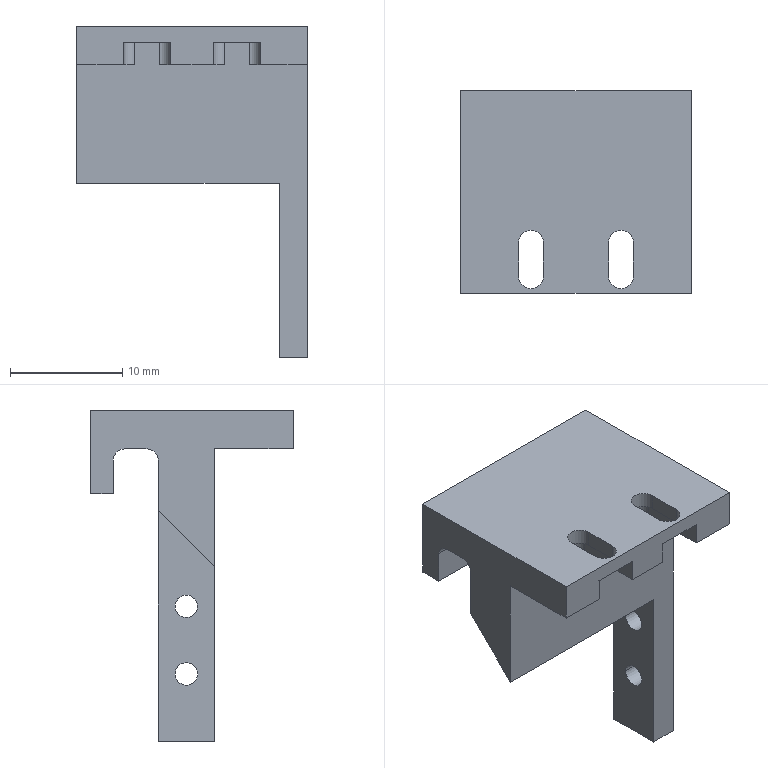NC program | NX | posted with a generic post | part box 20.5 x 18 x 29.4 mm
Lines 27 to 905 of 6588:
(ZLEVEL_PROFILE , TOOL : D10)
N52 T10 M6
N54 G54
N56 G17 G0 G90 X15.35 Y-7.488 S9500 M3
N58 G43 Z30. H10
N60 Z1.5
N62 G94 G1 Y-9.554 Z1.392 F1000.
N64 X15.016 Y-10.898 Z1.319
N66 X14.334 Y-12.104 Z1.247
N68 X13.354 Y-13.084 Z1.174
N70 X12.148 Y-13.766 Z1.101
N72 X10.804 Y-14.1 Z1.029
N74 X-10.804 Z-0.104
N76 X-12.148 Y-13.766 Z-0.176
N78 X-13.354 Y-13.084 Z-0.249
N80 X-14.334 Y-12.104 Z-0.322
N82 X-15.016 Y-10.898 Z-0.394
N84 X-15.35 Y-9.554 Z-0.467
N86 Y-9. Z-0.496
N88 Y9. F2500.
N90 G2 X-10.25 Y14.1 R5.1
N92 G1 X10.25
N94 G2 X15.35 Y9. R5.1
N96 G1 Y-9.
N98 G2 X10.25 Y-14.1 R5.1
N100 G1 X-10.25
N102 G2 X-15.35 Y-9. R5.1
N104 G1 Y8.655 Z-0.804
N106 Y9.039 Z-0.811
N108 X-15.332 Y9.423 Z-0.817
N110 X-15.286 Y9.804 Z-0.824
N112 X-15.212 Y10.18 Z-0.831
N114 X-15.109 Y10.55 Z-0.837
N116 X-14.979 Y10.911 Z-0.844
N118 X-14.822 Y11.261 Z-0.851
N120 X-14.639 Y11.598 Z-0.858
N122 X-14.431 Y11.921 Z-0.864
N124 X-14.199 Y12.227 Z-0.871
N126 X-13.946 Y12.515 Z-0.878
N128 X-13.671 Y12.782 Z-0.884
N130 X-13.377 Y13.029 Z-0.891
N132 X-13.065 Y13.253 Z-0.898
N134 X-12.737 Y13.452 Z-0.904
N136 X-12.396 Y13.627 Z-0.911
N138 X-12.042 Y13.775 Z-0.918
N140 X-11.678 Y13.896 Z-0.925
N142 X-11.305 Y13.99 Z-0.931
N144 X-10.927 Y14.055 Z-0.938
N146 X-10.545 Y14.091 Z-0.945
N148 X-10.162 Y14.1 Z-0.951
N150 X-7.859 Z-0.992
N152 X10.25
N154 G2 X15.35 Y9. R5.1
N156 G1 Y-9.
N158 G2 X10.25 Y-14.1 R5.1
N160 G1 X-10.25
N162 G2 X-15.35 Y-9. R5.1
N164 G1 Y8.655 Z-1.3
N166 Y9.039 Z-1.306
N168 X-15.332 Y9.423 Z-1.313
N170 X-15.286 Y9.804 Z-1.32
N172 X-15.212 Y10.18 Z-1.327
N174 X-15.109 Y10.55 Z-1.333
N176 X-14.979 Y10.911 Z-1.34
N178 X-14.822 Y11.261 Z-1.347
N180 X-14.639 Y11.598 Z-1.353
N182 X-14.431 Y11.921 Z-1.36
N184 X-14.199 Y12.227 Z-1.367
N186 X-13.946 Y12.515 Z-1.373
N188 X-13.671 Y12.782 Z-1.38
N190 X-13.377 Y13.029 Z-1.387
N192 X-13.065 Y13.253 Z-1.393
N194 X-12.737 Y13.452 Z-1.4
N196 X-12.396 Y13.627 Z-1.407
N198 X-12.042 Y13.775 Z-1.414
N200 X-11.678 Y13.896 Z-1.42
N202 X-11.305 Y13.99 Z-1.427
N204 X-10.927 Y14.055 Z-1.434
N206 X-10.545 Y14.091 Z-1.44
N208 X-10.162 Y14.1 Z-1.447
N210 X-7.859 Z-1.487
N212 X10.25
N214 G2 X15.35 Y9. R5.1
N216 G1 Y-9.
N218 G2 X10.25 Y-14.1 R5.1
N220 G1 X-10.25
N222 G2 X-15.35 Y-9. R5.1
N224 G1 Y8.655 Z-1.795
N226 Y9.039 Z-1.802
N228 X-15.332 Y9.423 Z-1.809
N230 X-15.286 Y9.804 Z-1.816
N232 X-15.212 Y10.18 Z-1.822
N234 X-15.109 Y10.55 Z-1.829
N236 X-14.979 Y10.911 Z-1.836
N238 X-14.822 Y11.261 Z-1.842
N240 X-14.639 Y11.598 Z-1.849
N242 X-14.431 Y11.921 Z-1.856
N244 X-14.199 Y12.227 Z-1.862
N246 X-13.946 Y12.515 Z-1.869
N248 X-13.671 Y12.782 Z-1.876
N250 X-13.377 Y13.029 Z-1.883
N252 X-13.065 Y13.253 Z-1.889
N254 X-12.737 Y13.452 Z-1.896
N256 X-12.396 Y13.627 Z-1.903
N258 X-12.042 Y13.775 Z-1.909
N260 X-11.678 Y13.896 Z-1.916
N262 X-11.305 Y13.99 Z-1.923
N264 X-10.927 Y14.055 Z-1.929
N266 X-10.545 Y14.091 Z-1.936
N268 X-10.162 Y14.1 Z-1.943
N270 X-7.859 Z-1.983
N272 X10.25
N274 G2 X15.35 Y9. R5.1
N276 G1 Y-9.
N278 G2 X10.25 Y-14.1 R5.1
N280 G1 X-10.25
N282 G2 X-15.35 Y-9. R5.1
N284 G1 Y8.655 Z-2.291
N286 Y9.039 Z-2.298
N288 X-15.332 Y9.423 Z-2.305
N290 X-15.286 Y9.804 Z-2.311
N292 X-15.212 Y10.18 Z-2.318
N294 X-15.109 Y10.55 Z-2.325
N296 X-14.979 Y10.911 Z-2.331
N298 X-14.822 Y11.261 Z-2.338
N300 X-14.639 Y11.598 Z-2.345
N302 X-14.431 Y11.921 Z-2.352
N304 X-14.199 Y12.227 Z-2.358
N306 X-13.946 Y12.515 Z-2.365
N308 X-13.671 Y12.782 Z-2.372
N310 X-13.377 Y13.029 Z-2.378
N312 X-13.065 Y13.253 Z-2.385
N314 X-12.737 Y13.452 Z-2.392
N316 X-12.396 Y13.627 Z-2.398
N318 X-12.042 Y13.775 Z-2.405
N320 X-11.678 Y13.896 Z-2.412
N322 X-11.305 Y13.99 Z-2.419
N324 X-10.927 Y14.055 Z-2.425
N326 X-10.545 Y14.091 Z-2.432
N328 X-10.162 Y14.1 Z-2.439
N330 X-7.859 Z-2.479
N332 X10.25
N334 G2 X15.35 Y9. R5.1
N336 G1 Y-9.
N338 G2 X10.25 Y-14.1 R5.1
N340 G1 X-10.25
N342 G2 X-15.35 Y-9. R5.1
N344 G1 Y8.655 Z-2.787
N346 Y9.039 Z-2.794
N348 X-15.332 Y9.423 Z-2.8
N350 X-15.286 Y9.804 Z-2.807
N352 X-15.212 Y10.18 Z-2.814
N354 X-15.109 Y10.55 Z-2.82
N356 X-14.979 Y10.911 Z-2.827
N358 X-14.822 Y11.261 Z-2.834
N360 X-14.639 Y11.598 Z-2.841
N362 X-14.431 Y11.921 Z-2.847
N364 X-14.199 Y12.227 Z-2.854
N366 X-13.946 Y12.515 Z-2.861
N368 X-13.671 Y12.782 Z-2.867
N370 X-13.377 Y13.029 Z-2.874
N372 X-13.065 Y13.253 Z-2.881
N374 X-12.737 Y13.452 Z-2.887
N376 X-12.396 Y13.627 Z-2.894
N378 X-12.042 Y13.775 Z-2.901
N380 X-11.678 Y13.896 Z-2.908
N382 X-11.305 Y13.99 Z-2.914
N384 X-10.927 Y14.055 Z-2.921
N386 X-10.545 Y14.091 Z-2.928
N388 X-10.162 Y14.1 Z-2.934
N390 X-7.859 Z-2.975
N392 X10.25
N394 G2 X15.35 Y9. R5.1
N396 G1 Y-9.
N398 G2 X10.25 Y-14.1 R5.1
N400 G1 X-10.25
N402 G2 X-15.35 Y-9. R5.1
N404 G1 Y8.655 Z-3.283
N406 Y9.039 Z-3.289
N408 X-15.332 Y9.423 Z-3.296
N410 X-15.286 Y9.804 Z-3.303
N412 X-15.212 Y10.18 Z-3.31
N414 X-15.109 Y10.55 Z-3.316
N416 X-14.979 Y10.911 Z-3.323
N418 X-14.822 Y11.261 Z-3.33
N420 X-14.639 Y11.598 Z-3.336
N422 X-14.431 Y11.921 Z-3.343
N424 X-14.199 Y12.227 Z-3.35
N426 X-13.946 Y12.515 Z-3.356
N428 X-13.671 Y12.782 Z-3.363
N430 X-13.377 Y13.029 Z-3.37
N432 X-13.065 Y13.253 Z-3.377
N434 X-12.737 Y13.452 Z-3.383
N436 X-12.396 Y13.627 Z-3.39
N438 X-12.042 Y13.775 Z-3.397
N440 X-11.678 Y13.896 Z-3.403
N442 X-11.305 Y13.99 Z-3.41
N444 X-10.927 Y14.055 Z-3.417
N446 X-10.545 Y14.091 Z-3.423
N448 X-10.162 Y14.1 Z-3.43
N450 X-7.859 Z-3.47
N452 X10.25
N454 G2 X15.35 Y9. R5.1
N456 G1 Y-9.
N458 G2 X10.25 Y-14.1 R5.1
N460 G1 X-10.25
N462 G2 X-15.35 Y-9. R5.1
N464 G1 Y8.655 Z-3.779
N466 Y9.039 Z-3.785
N468 X-15.332 Y9.423 Z-3.792
N470 X-15.286 Y9.804 Z-3.799
N472 X-15.212 Y10.18 Z-3.805
N474 X-15.109 Y10.55 Z-3.812
N476 X-14.979 Y10.911 Z-3.819
N478 X-14.822 Y11.261 Z-3.825
N480 X-14.639 Y11.598 Z-3.832
N482 X-14.431 Y11.921 Z-3.839
N484 X-14.199 Y12.227 Z-3.846
N486 X-13.946 Y12.515 Z-3.852
N488 X-13.671 Y12.782 Z-3.859
N490 X-13.377 Y13.029 Z-3.866
N492 X-13.065 Y13.253 Z-3.872
N494 X-12.737 Y13.452 Z-3.879
N496 X-12.396 Y13.627 Z-3.886
N498 X-12.042 Y13.775 Z-3.892
N500 X-11.678 Y13.896 Z-3.899
N502 X-11.305 Y13.99 Z-3.906
N504 X-10.927 Y14.055 Z-3.913
N506 X-10.545 Y14.091 Z-3.919
N508 X-10.162 Y14.1 Z-3.926
N510 X-7.859 Z-3.966
N512 X10.25
N514 G2 X15.35 Y9. R5.1
N516 G1 Y-9.
N518 G2 X10.25 Y-14.1 R5.1
N520 G1 X-10.25
N522 G2 X-15.35 Y-9. R5.1
N524 G1 Y8.655 Z-4.274
N526 Y9.039 Z-4.281
N528 X-15.332 Y9.423 Z-4.288
N530 X-15.286 Y9.804 Z-4.294
N532 X-15.212 Y10.18 Z-4.301
N534 X-15.109 Y10.55 Z-4.308
N536 X-14.979 Y10.911 Z-4.314
N538 X-14.822 Y11.261 Z-4.321
N540 X-14.639 Y11.598 Z-4.328
N542 X-14.431 Y11.921 Z-4.335
N544 X-14.199 Y12.227 Z-4.341
N546 X-13.946 Y12.515 Z-4.348
N548 X-13.671 Y12.782 Z-4.355
N550 X-13.377 Y13.029 Z-4.361
N552 X-13.065 Y13.253 Z-4.368
N554 X-12.737 Y13.452 Z-4.375
N556 X-12.396 Y13.627 Z-4.381
N558 X-12.042 Y13.775 Z-4.388
N560 X-11.678 Y13.896 Z-4.395
N562 X-11.305 Y13.99 Z-4.402
N564 X-10.927 Y14.055 Z-4.408
N566 X-10.545 Y14.091 Z-4.415
N568 X-10.162 Y14.1 Z-4.422
N570 X-7.859 Z-4.462
N572 X10.25
N574 G2 X15.35 Y9. R5.1
N576 G1 Y-9.
N578 G2 X10.25 Y-14.1 R5.1
N580 G1 X-10.25
N582 G2 X-15.35 Y-9. R5.1
N584 G1 Y8.655 Z-4.77
N586 Y9.039 Z-4.777
N588 X-15.332 Y9.423 Z-4.783
N590 X-15.286 Y9.804 Z-4.79
N592 X-15.212 Y10.18 Z-4.797
N594 X-15.109 Y10.55 Z-4.804
N596 X-14.979 Y10.911 Z-4.81
N598 X-14.822 Y11.261 Z-4.817
N600 X-14.639 Y11.598 Z-4.824
N602 X-14.431 Y11.921 Z-4.83
N604 X-14.199 Y12.227 Z-4.837
N606 X-13.946 Y12.515 Z-4.844
N608 X-13.671 Y12.782 Z-4.85
N610 X-13.377 Y13.029 Z-4.857
N612 X-13.065 Y13.253 Z-4.864
N614 X-12.737 Y13.452 Z-4.871
N616 X-12.396 Y13.627 Z-4.877
N618 X-12.042 Y13.775 Z-4.884
N620 X-11.678 Y13.896 Z-4.891
N622 X-11.305 Y13.99 Z-4.897
N624 X-10.927 Y14.055 Z-4.904
N626 X-10.545 Y14.091 Z-4.911
N628 X-10.162 Y14.1 Z-4.917
N630 X-7.859 Z-4.958
N632 X10.25
N634 G2 X15.35 Y9. R5.1
N636 G1 Y-9.
N638 G2 X10.25 Y-14.1 R5.1
N640 G1 X-10.25
N642 G2 X-15.35 Y-9. R5.1
N644 G1 Y8.655 Z-5.266
N646 Y9.039 Z-5.273
N648 X-15.332 Y9.423 Z-5.279
N650 X-15.286 Y9.804 Z-5.286
N652 X-15.212 Y10.18 Z-5.293
N654 X-15.109 Y10.55 Z-5.299
N656 X-14.979 Y10.911 Z-5.306
N658 X-14.822 Y11.261 Z-5.313
N660 X-14.639 Y11.598 Z-5.319
N662 X-14.431 Y11.921 Z-5.326
N664 X-14.199 Y12.227 Z-5.333
N666 X-13.946 Y12.515 Z-5.339
N668 X-13.671 Y12.782 Z-5.346
N670 X-13.377 Y13.029 Z-5.353
N672 X-13.065 Y13.253 Z-5.36
N674 X-12.737 Y13.452 Z-5.366
N676 X-12.396 Y13.627 Z-5.373
N678 X-12.042 Y13.775 Z-5.38
N680 X-11.678 Y13.896 Z-5.386
N682 X-11.305 Y13.99 Z-5.393
N684 X-10.927 Y14.055 Z-5.4
N686 X-10.545 Y14.091 Z-5.406
N688 X-10.162 Y14.1 Z-5.413
N690 X-7.859 Z-5.453
N692 X10.25
N694 G2 X15.35 Y9. R5.1
N696 G1 Y-9.
N698 G2 X10.25 Y-14.1 R5.1
N700 G1 X-10.25
N702 G2 X-15.35 Y-9. R5.1
N704 G1 Y8.655 Z-5.762
N706 Y9.039 Z-5.768
N708 X-15.332 Y9.423 Z-5.775
N710 X-15.286 Y9.804 Z-5.782
N712 X-15.212 Y10.18 Z-5.788
N714 X-15.109 Y10.55 Z-5.795
N716 X-14.979 Y10.911 Z-5.802
N718 X-14.822 Y11.261 Z-5.808
N720 X-14.639 Y11.598 Z-5.815
N722 X-14.431 Y11.921 Z-5.822
N724 X-14.199 Y12.227 Z-5.829
N726 X-13.946 Y12.515 Z-5.835
N728 X-13.671 Y12.782 Z-5.842
N730 X-13.377 Y13.029 Z-5.849
N732 X-13.065 Y13.253 Z-5.855
N734 X-12.737 Y13.452 Z-5.862
N736 X-12.396 Y13.627 Z-5.869
N738 X-12.042 Y13.775 Z-5.875
N740 X-11.678 Y13.896 Z-5.882
N742 X-11.305 Y13.99 Z-5.889
N744 X-10.927 Y14.055 Z-5.896
N746 X-10.545 Y14.091 Z-5.902
N748 X-10.162 Y14.1 Z-5.909
N750 X-7.859 Z-5.949
N752 X10.25
N754 G2 X15.35 Y9. R5.1
N756 G1 Y-9.
N758 G2 X10.25 Y-14.1 R5.1
N760 G1 X-10.25
N762 G2 X-15.35 Y-9. R5.1
N764 G1 Y8.655 Z-6.257
N766 Y9.039 Z-6.264
N768 X-15.332 Y9.423 Z-6.271
N770 X-15.286 Y9.804 Z-6.277
N772 X-15.212 Y10.18 Z-6.284
N774 X-15.109 Y10.55 Z-6.291
N776 X-14.979 Y10.911 Z-6.298
N778 X-14.822 Y11.261 Z-6.304
N780 X-14.639 Y11.598 Z-6.311
N782 X-14.431 Y11.921 Z-6.318
N784 X-14.199 Y12.227 Z-6.324
N786 X-13.946 Y12.515 Z-6.331
N788 X-13.671 Y12.782 Z-6.338
N790 X-13.377 Y13.029 Z-6.344
N792 X-13.065 Y13.253 Z-6.351
N794 X-12.737 Y13.452 Z-6.358
N796 X-12.396 Y13.627 Z-6.365
N798 X-12.042 Y13.775 Z-6.371
N800 X-11.678 Y13.896 Z-6.378
N802 X-11.305 Y13.99 Z-6.385
N804 X-10.927 Y14.055 Z-6.391
N806 X-10.545 Y14.091 Z-6.398
N808 X-10.162 Y14.1 Z-6.405
N810 X-7.859 Z-6.445
N812 X10.25
N814 G2 X15.35 Y9. R5.1
N816 G1 Y-9.
N818 G2 X10.25 Y-14.1 R5.1
N820 G1 X-10.25
N822 G2 X-15.35 Y-9. R5.1
N824 G1 Y8.655 Z-6.753
N826 Y9.039 Z-6.76
N828 X-15.332 Y9.423 Z-6.766
N830 X-15.286 Y9.804 Z-6.773
N832 X-15.212 Y10.18 Z-6.78
N834 X-15.109 Y10.55 Z-6.787
N836 X-14.979 Y10.911 Z-6.793
N838 X-14.822 Y11.261 Z-6.8
N840 X-14.639 Y11.598 Z-6.807
N842 X-14.431 Y11.921 Z-6.813
N844 X-14.199 Y12.227 Z-6.82
N846 X-13.946 Y12.515 Z-6.827
N848 X-13.671 Y12.782 Z-6.833
N850 X-13.377 Y13.029 Z-6.84
N852 X-13.065 Y13.253 Z-6.847
N854 X-12.737 Y13.452 Z-6.854
N856 X-12.396 Y13.627 Z-6.86
N858 X-12.042 Y13.775 Z-6.867
N860 X-11.678 Y13.896 Z-6.874
N862 X-11.305 Y13.99 Z-6.88
N864 X-10.927 Y14.055 Z-6.887
N866 X-10.545 Y14.091 Z-6.894
N868 X-10.162 Y14.1 Z-6.9
N870 X-7.859 Z-6.941
N872 X10.25
N874 G2 X15.35 Y9. R5.1
N876 G1 Y-9.
N878 G2 X10.25 Y-14.1 R5.1
N880 G1 X-10.25
N882 G2 X-15.35 Y-9. R5.1
N884 G1 Y8.655 Z-7.249
N886 Y9.039 Z-7.256
N888 X-15.332 Y9.423 Z-7.262
N890 X-15.286 Y9.804 Z-7.269
N892 X-15.212 Y10.18 Z-7.276
N894 X-15.109 Y10.55 Z-7.282
N896 X-14.979 Y10.911 Z-7.289
N898 X-14.822 Y11.261 Z-7.296
N900 X-14.639 Y11.598 Z-7.302
N902 X-14.431 Y11.921 Z-7.309
N904 X-14.199 Y12.227 Z-7.316
N906 X-13.946 Y12.515 Z-7.323
N908 X-13.671 Y12.782 Z-7.329
N910 X-13.377 Y13.029 Z-7.336
N912 X-13.065 Y13.253 Z-7.343
N914 X-12.737 Y13.452 Z-7.349
N916 X-12.396 Y13.627 Z-7.356
N918 X-12.042 Y13.775 Z-7.363
N920 X-11.678 Y13.896 Z-7.369
N922 X-11.305 Y13.99 Z-7.376
N924 X-10.927 Y14.055 Z-7.383
N926 X-10.545 Y14.091 Z-7.39
N928 X-10.162 Y14.1 Z-7.396
N930 X-7.859 Z-7.436
N932 X10.25
N934 G2 X15.35 Y9. R5.1
N936 G1 Y-9.
N938 G2 X10.25 Y-14.1 R5.1
N940 G1 X-10.25
N942 G2 X-15.35 Y-9. R5.1
N944 G1 Y8.655 Z-7.745
N946 Y9.039 Z-7.751
N948 X-15.332 Y9.423 Z-7.758
N950 X-15.286 Y9.804 Z-7.765
N952 X-15.212 Y10.18 Z-7.771
N954 X-15.109 Y10.55 Z-7.778
N956 X-14.979 Y10.911 Z-7.785
N958 X-14.822 Y11.261 Z-7.792
N960 X-14.639 Y11.598 Z-7.798
N962 X-14.431 Y11.921 Z-7.805
N964 X-14.199 Y12.227 Z-7.812
N966 X-13.946 Y12.515 Z-7.818
N968 X-13.671 Y12.782 Z-7.825
N970 X-13.377 Y13.029 Z-7.832
N972 X-13.065 Y13.253 Z-7.838
N974 X-12.737 Y13.452 Z-7.845
N976 X-12.396 Y13.627 Z-7.852
N978 X-12.042 Y13.775 Z-7.859
N980 X-11.678 Y13.896 Z-7.865
N982 X-11.305 Y13.99 Z-7.872
N984 X-10.927 Y14.055 Z-7.879
N986 X-10.545 Y14.091 Z-7.885
N988 X-10.162 Y14.1 Z-7.892
N990 X-7.859 Z-7.932
N992 X10.25
N994 G2 X15.35 Y9. R5.1
N996 G1 Y-9.
N998 G2 X10.25 Y-14.1 R5.1
N1000 G1 X-10.25
N1002 G2 X-15.35 Y-9. R5.1
N1004 G1 Y8.655 Z-8.24
N1006 Y9.039 Z-8.247
N1008 X-15.332 Y9.423 Z-8.254
N1010 X-15.286 Y9.804 Z-8.26
N1012 X-15.212 Y10.18 Z-8.267
N1014 X-15.109 Y10.55 Z-8.274
N1016 X-14.979 Y10.911 Z-8.281
N1018 X-14.822 Y11.261 Z-8.287
N1020 X-14.639 Y11.598 Z-8.294
N1022 X-14.431 Y11.921 Z-8.301
N1024 X-14.199 Y12.227 Z-8.307
N1026 X-13.946 Y12.515 Z-8.314
N1028 X-13.671 Y12.782 Z-8.321
N1030 X-13.377 Y13.029 Z-8.327
N1032 X-13.065 Y13.253 Z-8.334
N1034 X-12.737 Y13.452 Z-8.341
N1036 X-12.396 Y13.627 Z-8.348
N1038 X-12.042 Y13.775 Z-8.354
N1040 X-11.678 Y13.896 Z-8.361
N1042 X-11.305 Y13.99 Z-8.368
N1044 X-10.927 Y14.055 Z-8.374
N1046 X-10.545 Y14.091 Z-8.381
N1048 X-10.162 Y14.1 Z-8.388
N1050 X-7.859 Z-8.428
N1052 X10.25
N1054 G2 X15.35 Y9. R5.1
N1056 G1 Y-9.
N1058 G2 X10.25 Y-14.1 R5.1
N1060 G1 X-10.25
N1062 G2 X-15.35 Y-9. R5.1
N1064 G1 Y8.655 Z-8.736
N1066 Y9.039 Z-8.743
N1068 X-15.332 Y9.423 Z-8.75
N1070 X-15.286 Y9.804 Z-8.756
N1072 X-15.212 Y10.18 Z-8.763
N1074 X-15.109 Y10.55 Z-8.77
N1076 X-14.979 Y10.911 Z-8.776
N1078 X-14.822 Y11.261 Z-8.783
N1080 X-14.639 Y11.598 Z-8.79
N1082 X-14.431 Y11.921 Z-8.796
N1084 X-14.199 Y12.227 Z-8.803
N1086 X-13.946 Y12.515 Z-8.81
N1088 X-13.671 Y12.782 Z-8.817
N1090 X-13.377 Y13.029 Z-8.823
N1092 X-13.065 Y13.253 Z-8.83
N1094 X-12.737 Y13.452 Z-8.837
N1096 X-12.396 Y13.627 Z-8.843
N1098 X-12.042 Y13.775 Z-8.85
N1100 X-11.678 Y13.896 Z-8.857
N1102 X-11.305 Y13.99 Z-8.863
N1104 X-10.927 Y14.055 Z-8.87
N1106 X-10.545 Y14.091 Z-8.877
N1108 X-10.162 Y14.1 Z-8.884
N1110 X-7.859 Z-8.924
N1112 X10.25
N1114 G2 X15.35 Y9. R5.1
N1116 G1 Y-9.
N1118 G2 X10.25 Y-14.1 R5.1
N1120 G1 X-10.25
N1122 G2 X-15.35 Y-9. R5.1
N1124 G1 Y8.655 Z-9.232
N1126 Y9.039 Z-9.239
N1128 X-15.332 Y9.423 Z-9.245
N1130 X-15.286 Y9.804 Z-9.252
N1132 X-15.212 Y10.18 Z-9.259
N1134 X-15.109 Y10.55 Z-9.265
N1136 X-14.979 Y10.911 Z-9.272
N1138 X-14.822 Y11.261 Z-9.279
N1140 X-14.639 Y11.598 Z-9.286
N1142 X-14.431 Y11.921 Z-9.292
N1144 X-14.199 Y12.227 Z-9.299
N1146 X-13.946 Y12.515 Z-9.306
N1148 X-13.671 Y12.782 Z-9.312
N1150 X-13.377 Y13.029 Z-9.319
N1152 X-13.065 Y13.253 Z-9.326
N1154 X-12.737 Y13.452 Z-9.332
N1156 X-12.396 Y13.627 Z-9.339
N1158 X-12.042 Y13.775 Z-9.346
N1160 X-11.678 Y13.896 Z-9.352
N1162 X-11.305 Y13.99 Z-9.359
N1164 X-10.927 Y14.055 Z-9.366
N1166 X-10.545 Y14.091 Z-9.373
N1168 X-10.162 Y14.1 Z-9.379
N1170 X-7.859 Z-9.419
N1172 X10.25
N1174 G2 X15.35 Y9. R5.1
N1176 G1 Y-9.
N1178 G2 X10.25 Y-14.1 R5.1
N1180 G1 X-10.25
N1182 G2 X-15.35 Y-9. R5.1
N1184 G1 Y8.655 Z-9.728
N1186 Y9.039 Z-9.734
N1188 X-15.332 Y9.423 Z-9.741
N1190 X-15.286 Y9.804 Z-9.748
N1192 X-15.212 Y10.18 Z-9.754
N1194 X-15.109 Y10.55 Z-9.761
N1196 X-14.979 Y10.911 Z-9.768
N1198 X-14.822 Y11.261 Z-9.775
N1200 X-14.639 Y11.598 Z-9.781
N1202 X-14.431 Y11.921 Z-9.788
N1204 X-14.199 Y12.227 Z-9.795
N1206 X-13.946 Y12.515 Z-9.801
N1208 X-13.671 Y12.782 Z-9.808
N1210 X-13.377 Y13.029 Z-9.815
N1212 X-13.065 Y13.253 Z-9.821
N1214 X-12.737 Y13.452 Z-9.828
N1216 X-12.396 Y13.627 Z-9.835
N1218 X-12.042 Y13.775 Z-9.842
N1220 X-11.678 Y13.896 Z-9.848
N1222 X-11.305 Y13.99 Z-9.855
N1224 X-10.927 Y14.055 Z-9.862
N1226 X-10.545 Y14.091 Z-9.868
N1228 X-10.162 Y14.1 Z-9.875
N1230 X-7.859 Z-9.915
N1232 X10.25
N1234 G2 X15.35 Y9. R5.1
N1236 G1 Y-9.
N1238 G2 X10.25 Y-14.1 R5.1
N1240 G1 X-10.25
N1242 G2 X-15.35 Y-9. R5.1
N1244 G1 Y8.655 Z-10.223
N1246 Y9.039 Z-10.23
N1248 X-15.332 Y9.423 Z-10.237
N1250 X-15.286 Y9.804 Z-10.244
N1252 X-15.212 Y10.18 Z-10.25
N1254 X-15.109 Y10.55 Z-10.257
N1256 X-14.979 Y10.911 Z-10.264
N1258 X-14.822 Y11.261 Z-10.27
N1260 X-14.639 Y11.598 Z-10.277
N1262 X-14.431 Y11.921 Z-10.284
N1264 X-14.199 Y12.227 Z-10.29
N1266 X-13.946 Y12.515 Z-10.297
N1268 X-13.671 Y12.782 Z-10.304
N1270 X-13.377 Y13.029 Z-10.311
N1272 X-13.065 Y13.253 Z-10.317
N1274 X-12.737 Y13.452 Z-10.324
N1276 X-12.396 Y13.627 Z-10.331
N1278 X-12.042 Y13.775 Z-10.337
N1280 X-11.678 Y13.896 Z-10.344
N1282 X-11.305 Y13.99 Z-10.351
N1284 X-10.927 Y14.055 Z-10.357
N1286 X-10.545 Y14.091 Z-10.364
N1288 X-10.162 Y14.1 Z-10.371
N1290 X-7.859 Z-10.411
N1292 X10.25
N1294 G2 X15.35 Y9. R5.1
N1296 G1 Y-9.
N1298 G2 X10.25 Y-14.1 R5.1
N1300 G1 X-10.25
N1302 G2 X-15.35 Y-9. R5.1
N1304 G1 Y8.655 Z-10.719
N1306 Y9.039 Z-10.726
N1308 X-15.332 Y9.423 Z-10.733
N1310 X-15.286 Y9.804 Z-10.739
N1312 X-15.212 Y10.18 Z-10.746
N1314 X-15.109 Y10.55 Z-10.753
N1316 X-14.979 Y10.911 Z-10.759
N1318 X-14.822 Y11.261 Z-10.766
N1320 X-14.639 Y11.598 Z-10.773
N1322 X-14.431 Y11.921 Z-10.779
N1324 X-14.199 Y12.227 Z-10.786
N1326 X-13.946 Y12.515 Z-10.793
N1328 X-13.671 Y12.782 Z-10.8
N1330 X-13.377 Y13.029 Z-10.806
N1332 X-13.065 Y13.253 Z-10.813
N1334 X-12.737 Y13.452 Z-10.82
N1336 X-12.396 Y13.627 Z-10.826
N1338 X-12.042 Y13.775 Z-10.833
N1340 X-11.678 Y13.896 Z-10.84
N1342 X-11.305 Y13.99 Z-10.846
N1344 X-10.927 Y14.055 Z-10.853
N1346 X-10.545 Y14.091 Z-10.86
N1348 X-10.162 Y14.1 Z-10.867
N1350 X-7.859 Z-10.907
N1352 X10.25
N1354 G2 X15.35 Y9. R5.1
N1356 G1 Y-9.
N1358 G2 X10.25 Y-14.1 R5.1
N1360 G1 X-10.25
N1362 G2 X-15.35 Y-9. R5.1
N1364 G1 Y8.655 Z-11.215
N1366 Y9.039 Z-11.222
N1368 X-15.332 Y9.423 Z-11.228
N1370 X-15.286 Y9.804 Z-11.235
N1372 X-15.212 Y10.18 Z-11.242
N1374 X-15.109 Y10.55 Z-11.248
N1376 X-14.979 Y10.911 Z-11.255
N1378 X-14.822 Y11.261 Z-11.262
N1380 X-14.639 Y11.598 Z-11.269
N1382 X-14.431 Y11.921 Z-11.275
N1384 X-14.199 Y12.227 Z-11.282
N1386 X-13.946 Y12.515 Z-11.289
N1388 X-13.671 Y12.782 Z-11.295
N1390 X-13.377 Y13.029 Z-11.302
N1392 X-13.065 Y13.253 Z-11.309
N1394 X-12.737 Y13.452 Z-11.315
N1396 X-12.396 Y13.627 Z-11.322
N1398 X-12.042 Y13.775 Z-11.329
N1400 X-11.678 Y13.896 Z-11.336
N1402 X-11.305 Y13.99 Z-11.342
N1404 X-10.927 Y14.055 Z-11.349
N1406 X-10.545 Y14.091 Z-11.356
N1408 X-10.162 Y14.1 Z-11.362
N1410 X-7.859 Z-11.403
N1412 X10.25
N1414 G2 X15.35 Y9. R5.1
N1416 G1 Y-9.
N1418 G2 X10.25 Y-14.1 R5.1
N1420 G1 X-10.25
N1422 G2 X-15.35 Y-9. R5.1
N1424 G1 Y8.655 Z-11.711
N1426 Y9.039 Z-11.717
N1428 X-15.332 Y9.423 Z-11.724
N1430 X-15.286 Y9.804 Z-11.731
N1432 X-15.212 Y10.18 Z-11.738
N1434 X-15.109 Y10.55 Z-11.744
N1436 X-14.979 Y10.911 Z-11.751
N1438 X-14.822 Y11.261 Z-11.758
N1440 X-14.639 Y11.598 Z-11.764
N1442 X-14.431 Y11.921 Z-11.771
N1444 X-14.199 Y12.227 Z-11.778
N1446 X-13.946 Y12.515 Z-11.784
N1448 X-13.671 Y12.782 Z-11.791
N1450 X-13.377 Y13.029 Z-11.798
N1452 X-13.065 Y13.253 Z-11.805
N1454 X-12.737 Y13.452 Z-11.811
N1456 X-12.396 Y13.627 Z-11.818
N1458 X-12.042 Y13.775 Z-11.825
N1460 X-11.678 Y13.896 Z-11.831
N1462 X-11.305 Y13.99 Z-11.838
N1464 X-10.927 Y14.055 Z-11.845
N1466 X-10.545 Y14.091 Z-11.851
N1468 X-10.162 Y14.1 Z-11.858
N1470 X-7.859 Z-11.898
N1472 X10.25
N1474 G2 X15.35 Y9. R5.1
N1476 G1 Y-9.
N1478 G2 X10.25 Y-14.1 R5.1
N1480 G1 X-10.25
N1482 G2 X-15.35 Y-9. R5.1
N1484 G1 Y8.655 Z-12.206
N1486 Y9.039 Z-12.213
N1488 X-15.332 Y9.423 Z-12.22
N1490 X-15.286 Y9.804 Z-12.227
N1492 X-15.212 Y10.18 Z-12.233
N1494 X-15.109 Y10.55 Z-12.24
N1496 X-14.979 Y10.911 Z-12.247
N1498 X-14.822 Y11.261 Z-12.253
N1500 X-14.639 Y11.598 Z-12.26
N1502 X-14.431 Y11.921 Z-12.267
N1504 X-14.199 Y12.227 Z-12.273
N1506 X-13.946 Y12.515 Z-12.28
N1508 X-13.671 Y12.782 Z-12.287
N1510 X-13.377 Y13.029 Z-12.294
N1512 X-13.065 Y13.253 Z-12.3
N1514 X-12.737 Y13.452 Z-12.307
N1516 X-12.396 Y13.627 Z-12.314
N1518 X-12.042 Y13.775 Z-12.32
N1520 X-11.678 Y13.896 Z-12.327
N1522 X-11.305 Y13.99 Z-12.334
N1524 X-10.927 Y14.055 Z-12.34
N1526 X-10.545 Y14.091 Z-12.347
N1528 X-10.162 Y14.1 Z-12.354
N1530 X-7.859 Z-12.394
N1532 X10.25
N1534 G2 X15.35 Y9. R5.1
N1536 G1 Y-9.
N1538 G2 X10.25 Y-14.1 R5.1
N1540 G1 X-10.25
N1542 G2 X-15.35 Y-9. R5.1
N1544 G1 Y8.655 Z-12.702
N1546 Y9.039 Z-12.709
N1548 X-15.332 Y9.423 Z-12.716
N1550 X-15.286 Y9.804 Z-12.722
N1552 X-15.212 Y10.18 Z-12.729
N1554 X-15.109 Y10.55 Z-12.736
N1556 X-14.979 Y10.911 Z-12.742
N1558 X-14.822 Y11.261 Z-12.749
N1560 X-14.639 Y11.598 Z-12.756
N1562 X-14.431 Y11.921 Z-12.763
N1564 X-14.199 Y12.227 Z-12.769
N1566 X-13.946 Y12.515 Z-12.776
N1568 X-13.671 Y12.782 Z-12.783
N1570 X-13.377 Y13.029 Z-12.789
N1572 X-13.065 Y13.253 Z-12.796
N1574 X-12.737 Y13.452 Z-12.803
N1576 X-12.396 Y13.627 Z-12.809
N1578 X-12.042 Y13.775 Z-12.816
N1580 X-11.678 Y13.896 Z-12.823
N1582 X-11.305 Y13.99 Z-12.83
N1584 X-10.927 Y14.055 Z-12.836
N1586 X-10.545 Y14.091 Z-12.843
N1588 X-10.162 Y14.1 Z-12.85
N1590 X-7.859 Z-12.89
N1592 X10.25
N1594 G2 X15.35 Y9. R5.1
N1596 G1 Y-9.
N1598 G2 X10.25 Y-14.1 R5.1
N1600 G1 X-10.25
N1602 G2 X-15.35 Y-9. R5.1
N1604 G1 Y8.655 Z-13.198
N1606 Y9.039 Z-13.205
N1608 X-15.332 Y9.423 Z-13.211
N1610 X-15.286 Y9.804 Z-13.218
N1612 X-15.212 Y10.18 Z-13.225
N1614 X-15.109 Y10.55 Z-13.232
N1616 X-14.979 Y10.911 Z-13.238
N1618 X-14.822 Y11.261 Z-13.245
N1620 X-14.639 Y11.598 Z-13.252
N1622 X-14.431 Y11.921 Z-13.258
N1624 X-14.199 Y12.227 Z-13.265
N1626 X-13.946 Y12.515 Z-13.272
N1628 X-13.671 Y12.782 Z-13.278
N1630 X-13.377 Y13.029 Z-13.285
N1632 X-13.065 Y13.253 Z-13.292
N1634 X-12.737 Y13.452 Z-13.299
N1636 X-12.396 Y13.627 Z-13.305
N1638 X-12.042 Y13.775 Z-13.312
N1640 X-11.678 Y13.896 Z-13.319
N1642 X-11.305 Y13.99 Z-13.325
N1644 X-10.927 Y14.055 Z-13.332
N1646 X-10.545 Y14.091 Z-13.339
N1648 X-10.162 Y14.1 Z-13.345
N1650 X-7.859 Z-13.386
N1652 X10.25
N1654 G2 X15.35 Y9. R5.1
N1656 G1 Y-9.
N1658 G2 X10.25 Y-14.1 R5.1
N1660 G1 X-10.25
N1662 G2 X-15.35 Y-9. R5.1
N1664 G1 Y8.655 Z-13.694
N1666 Y9.039 Z-13.7
N1668 X-15.332 Y9.423 Z-13.707
N1670 X-15.286 Y9.804 Z-13.714
N1672 X-15.212 Y10.18 Z-13.721
N1674 X-15.109 Y10.55 Z-13.727
N1676 X-14.979 Y10.911 Z-13.734
N1678 X-14.822 Y11.261 Z-13.741
N1680 X-14.639 Y11.598 Z-13.747
N1682 X-14.431 Y11.921 Z-13.754
N1684 X-14.199 Y12.227 Z-13.761
N1686 X-13.946 Y12.515 Z-13.767
N1688 X-13.671 Y12.782 Z-13.774
N1690 X-13.377 Y13.029 Z-13.781
N1692 X-13.065 Y13.253 Z-13.788
N1694 X-12.737 Y13.452 Z-13.794
N1696 X-12.396 Y13.627 Z-13.801
N1698 X-12.042 Y13.775 Z-13.808
N1700 X-11.678 Y13.896 Z-13.814
N1702 X-11.305 Y13.99 Z-13.821
N1704 X-10.927 Y14.055 Z-13.828
N1706 X-10.545 Y14.091 Z-13.834
N1708 X-10.162 Y14.1 Z-13.841
N1710 X-7.859 Z-13.881
N1712 X10.25
N1714 G2 X15.35 Y9. R5.1
N1716 G1 Y-9.
N1718 G2 X10.25 Y-14.1 R5.1
N1720 G1 X-10.25
N1722 G2 X-15.35 Y-9. R5.1
N1724 G1 Y8.655 Z-14.19
N1726 Y9.039 Z-14.196
N1728 X-15.332 Y9.423 Z-14.203
N1730 X-15.286 Y9.804 Z-14.21
N1732 X-15.212 Y10.18 Z-14.216
N1734 X-15.109 Y10.55 Z-14.223
N1736 X-14.979 Y10.911 Z-14.23
N1738 X-14.822 Y11.261 Z-14.236
N1740 X-14.639 Y11.598 Z-14.243
N1742 X-14.431 Y11.921 Z-14.25
N1744 X-14.199 Y12.227 Z-14.257
N1746 X-13.946 Y12.515 Z-14.263
N1748 X-13.671 Y12.782 Z-14.27
N1750 X-13.377 Y13.029 Z-14.277
N1752 X-13.065 Y13.253 Z-14.283
N1754 X-12.737 Y13.452 Z-14.29
N1756 X-12.396 Y13.627 Z-14.297
N1758 X-12.042 Y13.775 Z-14.303
N1760 X-11.678 Y13.896 Z-14.31
N1762 X-11.305 Y13.99 Z-14.317
N1764 X-10.927 Y14.055 Z-14.324
N1766 X-10.545 Y14.091 Z-14.33
N1768 X-10.162 Y14.1 Z-14.337
N1770 X-7.859 Z-14.377
N1772 X10.25
N1774 G2 X15.35 Y9. R5.1
N1776 G1 Y-9.
N1778 G2 X10.25 Y-14.1 R5.1
N1780 G1 X-10.25
N1782 G2 X-15.35 Y-9. R5.1
N1784 G1 Y8.655 Z-14.685
N1786 Y9.039 Z-14.692
N1788 X-15.332 Y9.423 Z-14.699
N1790 X-15.286 Y9.804 Z-14.705
N1792 X-15.212 Y10.18 Z-14.712
N1794 X-15.109 Y10.55 Z-14.719
N1796 X-14.979 Y10.911 Z-14.725
N1798 X-14.822 Y11.261 Z-14.732
N1800 X-14.639 Y11.598 Z-14.739
N1802 X-14.431 Y11.921 Z-14.746